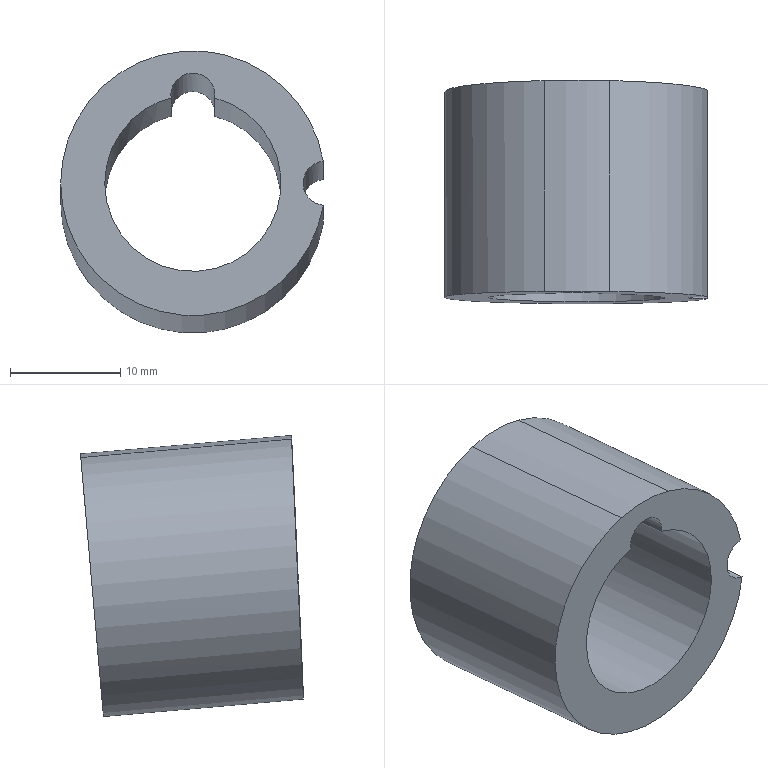Part | NX | features solid 2 | 1 solid | 8 faces | box 23.833 x 20.243 x 25.583 mm | volume 4465 mm3 | cylinder 5 | plane 2 | spline 1 | commonest cylinder face diameters 4 x2 24 x2 16 x1
STEP:
#1=CARTESIAN_POINT('',(201.703,-46.311,-35.578));
#2=VERTEX_POINT('',#1);
#3=CARTESIAN_POINT('',(210.56,-46.767,-45.207));
#4=VERTEX_POINT('',#3);
#5=CARTESIAN_POINT('',(198.727,-46.835,-47.202));
#6=DIRECTION('',(0.001957,0.999,-0.04546));
#7=DIRECTION('',(0.04675,0.04532,0.9979));
#8=AXIS2_PLACEMENT_3D('',#5,#6,#7);
#9=ELLIPSE('',#8,12.011,12.);
#10=EDGE_CURVE('',#2,#4,#9,.T.);
#11=ORIENTED_EDGE('',*,*,#10,.T.);
#12=CARTESIAN_POINT('',(210.56,-28.01,-46.848));
#13=VERTEX_POINT('',#12);
#14=CARTESIAN_POINT('',(210.56,-37.445,-46.023));
#15=DIRECTION('',(0.,0.9962,-0.08716));
#16=VECTOR('',#15,1000.);
#17=LINE('',#14,#16);
#18=EDGE_CURVE('',#4,#13,#17,.T.);
#19=ORIENTED_EDGE('',*,*,#18,.T.);
#20=CARTESIAN_POINT('',(201.703,-27.17,-37.253));
#21=VERTEX_POINT('',#20);
#22=CARTESIAN_POINT('',(198.727,-28.184,-48.834));
#23=DIRECTION('',(0.,0.9962,-0.08716));
#24=DIRECTION('',(0.,0.08716,0.9962));
#25=AXIS2_PLACEMENT_3D('',#22,#23,#24);
#26=CIRCLE('',#25,12.);
#27=EDGE_CURVE('',#21,#13,#26,.T.);
#28=ORIENTED_EDGE('',*,*,#27,.F.);
#29=CARTESIAN_POINT('',(201.703,-27.17,-37.253));
#30=DIRECTION('',(0.,-0.9962,0.08716));
#31=VECTOR('',#30,1000.);
#32=LINE('',#29,#31);
#33=EDGE_CURVE('',#21,#2,#32,.T.);
#34=ORIENTED_EDGE('',*,*,#33,.T.);
#35=EDGE_LOOP('',(#11,#19,#28,#34));
#36=FACE_BOUND('',#35,.T.);
#37=CARTESIAN_POINT('',(198.727,-28.184,-48.834));
#38=DIRECTION('',(0.,-0.9962,0.08716));
#39=DIRECTION('',(0.,-0.08716,-0.9962));
#40=AXIS2_PLACEMENT_3D('',#37,#38,#39);
#41=CYLINDRICAL_SURFACE('',#40,12.);
#42=ADVANCED_FACE('',(#36),#41,.T.);
#43=CARTESIAN_POINT('',(200.711,-46.486,-39.453));
#44=VERTEX_POINT('',#43);
#45=CARTESIAN_POINT('',(196.742,-46.478,-39.454));
#46=VERTEX_POINT('',#45);
#47=CARTESIAN_POINT('',(198.727,-46.835,-47.202));
#48=DIRECTION('',(0.001957,0.999,-0.04546));
#49=DIRECTION('',(0.04675,0.04532,0.9979));
#50=AXIS2_PLACEMENT_3D('',#47,#48,#49);
#51=ELLIPSE('',#50,8.007,8.);
#52=EDGE_CURVE('',#44,#46,#51,.T.);
#53=ORIENTED_EDGE('',*,*,#52,.F.);
#54=CARTESIAN_POINT('',(200.711,-27.508,-41.113));
#55=VERTEX_POINT('',#54);
#56=CARTESIAN_POINT('',(200.711,-27.508,-41.113));
#57=DIRECTION('',(0.,-0.9962,0.08716));
#58=VECTOR('',#57,1000.);
#59=LINE('',#56,#58);
#60=EDGE_CURVE('',#44,#55,#59,.F.);
#61=ORIENTED_EDGE('',*,*,#60,.T.);
#62=CARTESIAN_POINT('',(196.742,-27.508,-41.113));
#63=VERTEX_POINT('',#62);
#64=CARTESIAN_POINT('',(198.727,-28.184,-48.834));
#65=DIRECTION('',(0.,-0.9962,0.08716));
#66=DIRECTION('',(0.,-0.08716,-0.9962));
#67=AXIS2_PLACEMENT_3D('',#64,#65,#66);
#68=CIRCLE('',#67,8.);
#69=EDGE_CURVE('',#55,#63,#68,.F.);
#70=ORIENTED_EDGE('',*,*,#69,.T.);
#71=CARTESIAN_POINT('',(196.742,-27.508,-41.113));
#72=DIRECTION('',(0.,-0.9962,0.08716));
#73=VECTOR('',#72,1000.);
#74=LINE('',#71,#73);
#75=EDGE_CURVE('',#63,#46,#74,.T.);
#76=ORIENTED_EDGE('',*,*,#75,.T.);
#77=EDGE_LOOP('',(#53,#61,#70,#76));
#78=FACE_BOUND('',#77,.T.);
#79=CARTESIAN_POINT('',(198.727,-28.184,-48.834));
#80=DIRECTION('',(0.,-0.9962,0.08716));
#81=DIRECTION('',(0.,-0.08716,-0.9962));
#82=AXIS2_PLACEMENT_3D('',#79,#80,#81);
#83=CYLINDRICAL_SURFACE('',#82,8.);
#84=ADVANCED_FACE('',(#78),#83,.F.);
#85=CARTESIAN_POINT('',(210.56,-28.357,-50.819));
#86=VERTEX_POINT('',#85);
#87=CARTESIAN_POINT('',(210.727,-28.184,-48.834));
#88=DIRECTION('',(0.,-0.9962,0.08716));
#89=DIRECTION('',(0.,-0.08716,-0.9962));
#90=AXIS2_PLACEMENT_3D('',#87,#88,#89);
#91=CIRCLE('',#90,2.);
#92=EDGE_CURVE('',#13,#86,#91,.T.);
#93=ORIENTED_EDGE('',*,*,#92,.T.);
#94=CARTESIAN_POINT('',(195.75,-27.17,-37.253));
#95=VERTEX_POINT('',#94);
#96=CARTESIAN_POINT('',(198.727,-28.184,-48.834));
#97=DIRECTION('',(0.,0.9962,-0.08716));
#98=DIRECTION('',(0.,0.08716,0.9962));
#99=AXIS2_PLACEMENT_3D('',#96,#97,#98);
#100=CIRCLE('',#99,12.);
#101=EDGE_CURVE('',#86,#95,#100,.T.);
#102=ORIENTED_EDGE('',*,*,#101,.T.);
#103=CARTESIAN_POINT('',(195.75,-27.17,-37.253));
#104=CARTESIAN_POINT('',(197.703,-27.127,-36.755));
#105=CARTESIAN_POINT('',(199.75,-27.127,-36.755));
#106=CARTESIAN_POINT('',(201.703,-27.17,-37.253));
#107=B_SPLINE_CURVE_WITH_KNOTS('',3,(#103,#104,#105,#106),.UNSPECIFIED.,.F.,.F.,(4,4),(0.,1.),.PIECEWISE_BEZIER_KNOTS.);
#108=EDGE_CURVE('',#95,#21,#107,.T.);
#109=ORIENTED_EDGE('',*,*,#108,.T.);
#110=ORIENTED_EDGE('',*,*,#27,.T.);
#111=EDGE_LOOP('',(#93,#102,#109,#110));
#112=FACE_BOUND('',#111,.T.);
#113=CARTESIAN_POINT('',(198.727,-27.486,-40.864));
#114=DIRECTION('',(0.,-0.9962,0.08716));
#115=DIRECTION('',(0.,-0.08716,-0.9962));
#116=AXIS2_PLACEMENT_3D('',#113,#114,#115);
#117=CIRCLE('',#116,2.);
#118=EDGE_CURVE('',#55,#63,#117,.T.);
#119=ORIENTED_EDGE('',*,*,#118,.T.);
#120=ORIENTED_EDGE('',*,*,#69,.F.);
#121=EDGE_LOOP('',(#119,#120));
#122=FACE_BOUND('',#121,.T.);
#123=CARTESIAN_POINT('',(195.75,-27.17,-37.253));
#124=DIRECTION('',(0.,0.9962,-0.08716));
#125=DIRECTION('',(0.,0.08716,0.9962));
#126=AXIS2_PLACEMENT_3D('',#123,#124,#125);
#127=PLANE('',#126);
#128=ADVANCED_FACE('',(#112,#122),#127,.T.);
#129=CARTESIAN_POINT('',(210.56,-46.948,-49.193));
#130=VERTEX_POINT('',#129);
#131=CARTESIAN_POINT('',(210.727,-46.858,-47.2));
#132=DIRECTION('',(0.001957,0.999,-0.04546));
#133=DIRECTION('',(-0.04675,-0.04532,-0.9979));
#134=AXIS2_PLACEMENT_3D('',#131,#132,#133);
#135=ELLIPSE('',#134,2.002,2.);
#136=EDGE_CURVE('',#130,#4,#135,.T.);
#137=ORIENTED_EDGE('',*,*,#136,.T.);
#138=ORIENTED_EDGE('',*,*,#10,.F.);
#139=CARTESIAN_POINT('',(195.75,-46.3,-35.579));
#140=VERTEX_POINT('',#139);
#141=CARTESIAN_POINT('',(195.75,-46.3,-35.579));
#142=CARTESIAN_POINT('',(197.699,-46.281,-35.08));
#143=CARTESIAN_POINT('',(199.754,-46.285,-35.08));
#144=CARTESIAN_POINT('',(201.703,-46.311,-35.578));
#145=B_SPLINE_CURVE_WITH_KNOTS('',3,(#141,#142,#143,#144),.UNSPECIFIED.,.F.,.F.,(4,4),(0.,0.006022),.UNSPECIFIED.);
#146=EDGE_CURVE('',#140,#2,#145,.T.);
#147=ORIENTED_EDGE('',*,*,#146,.F.);
#148=CARTESIAN_POINT('',(198.727,-46.835,-47.202));
#149=DIRECTION('',(0.001957,0.999,-0.04546));
#150=DIRECTION('',(0.04675,0.04532,0.9979));
#151=AXIS2_PLACEMENT_3D('',#148,#149,#150);
#152=ELLIPSE('',#151,12.011,12.);
#153=EDGE_CURVE('',#130,#140,#152,.T.);
#154=ORIENTED_EDGE('',*,*,#153,.F.);
#155=EDGE_LOOP('',(#137,#138,#147,#154));
#156=FACE_BOUND('',#155,.T.);
#157=CARTESIAN_POINT('',(198.727,-46.471,-39.203));
#158=DIRECTION('',(0.001957,0.999,-0.04546));
#159=DIRECTION('',(-0.04675,-0.04532,-0.9979));
#160=AXIS2_PLACEMENT_3D('',#157,#158,#159);
#161=ELLIPSE('',#160,2.002,2.);
#162=EDGE_CURVE('',#46,#44,#161,.T.);
#163=ORIENTED_EDGE('',*,*,#162,.T.);
#164=ORIENTED_EDGE('',*,*,#52,.T.);
#165=EDGE_LOOP('',(#163,#164));
#166=FACE_BOUND('',#165,.T.);
#167=CARTESIAN_POINT('',(128.811,-48.589,-88.763));
#168=DIRECTION('',(0.001957,0.999,-0.04546));
#169=DIRECTION('',(0.06617,0.04523,0.9968));
#170=AXIS2_PLACEMENT_3D('',#167,#168,#169);
#171=PLANE('',#170);
#172=ADVANCED_FACE('',(#156,#166),#171,.F.);
#173=ORIENTED_EDGE('',*,*,#101,.F.);
#174=CARTESIAN_POINT('',(210.56,-37.792,-49.994));
#175=DIRECTION('',(0.,0.9962,-0.08716));
#176=VECTOR('',#175,1000.);
#177=LINE('',#174,#176);
#178=EDGE_CURVE('',#86,#130,#177,.F.);
#179=ORIENTED_EDGE('',*,*,#178,.T.);
#180=ORIENTED_EDGE('',*,*,#153,.T.);
#181=CARTESIAN_POINT('',(195.75,-27.17,-37.253));
#182=DIRECTION('',(0.,-0.9962,0.08716));
#183=VECTOR('',#182,1000.);
#184=LINE('',#181,#183);
#185=EDGE_CURVE('',#95,#140,#184,.T.);
#186=ORIENTED_EDGE('',*,*,#185,.F.);
#187=EDGE_LOOP('',(#173,#179,#180,#186));
#188=FACE_BOUND('',#187,.T.);
#189=CARTESIAN_POINT('',(198.727,-28.184,-48.834));
#190=DIRECTION('',(0.,-0.9962,0.08716));
#191=DIRECTION('',(0.,-0.08716,-0.9962));
#192=AXIS2_PLACEMENT_3D('',#189,#190,#191);
#193=CYLINDRICAL_SURFACE('',#192,12.);
#194=ADVANCED_FACE('',(#188),#193,.T.);
#195=ORIENTED_EDGE('',*,*,#146,.T.);
#196=ORIENTED_EDGE('',*,*,#33,.F.);
#197=ORIENTED_EDGE('',*,*,#108,.F.);
#198=ORIENTED_EDGE('',*,*,#185,.T.);
#199=EDGE_LOOP('',(#195,#196,#197,#198));
#200=FACE_BOUND('',#199,.T.);
#201=CARTESIAN_POINT('',(195.75,-27.17,-37.253));
#202=CARTESIAN_POINT('',(195.75,-46.438,-35.567));
#203=CARTESIAN_POINT('',(197.703,-27.127,-36.755));
#204=CARTESIAN_POINT('',(197.703,-46.394,-35.069));
#205=CARTESIAN_POINT('',(199.75,-27.127,-36.755));
#206=CARTESIAN_POINT('',(199.75,-46.394,-35.069));
#207=CARTESIAN_POINT('',(201.703,-27.17,-37.253));
#208=CARTESIAN_POINT('',(201.703,-46.438,-35.567));
#209=B_SPLINE_SURFACE_WITH_KNOTS('',3,1,((#201,#202),(#203,#204),(#205,#206),(#207,#208)),.SURF_OF_LINEAR_EXTRUSION.,.F.,.F.,.F.,(4,4),(2,2),(0.,1.),(0.,1.),.PIECEWISE_BEZIER_KNOTS.);
#210=ADVANCED_FACE('',(#200),#209,.F.);
#211=ORIENTED_EDGE('',*,*,#75,.F.);
#212=ORIENTED_EDGE('',*,*,#118,.F.);
#213=ORIENTED_EDGE('',*,*,#60,.F.);
#214=ORIENTED_EDGE('',*,*,#162,.F.);
#215=EDGE_LOOP('',(#211,#212,#213,#214));
#216=FACE_BOUND('',#215,.T.);
#217=CARTESIAN_POINT('',(198.727,-47.41,-39.121));
#218=DIRECTION('',(0.,0.9962,-0.08716));
#219=DIRECTION('',(0.,0.08716,0.9962));
#220=AXIS2_PLACEMENT_3D('',#217,#218,#219);
#221=CYLINDRICAL_SURFACE('',#220,2.);
#222=ADVANCED_FACE('',(#216),#221,.F.);
#223=ORIENTED_EDGE('',*,*,#136,.F.);
#224=ORIENTED_EDGE('',*,*,#178,.F.);
#225=ORIENTED_EDGE('',*,*,#92,.F.);
#226=ORIENTED_EDGE('',*,*,#18,.F.);
#227=EDGE_LOOP('',(#223,#224,#225,#226));
#228=FACE_BOUND('',#227,.T.);
#229=CARTESIAN_POINT('',(210.727,-48.107,-47.091));
#230=DIRECTION('',(0.,0.9962,-0.08716));
#231=DIRECTION('',(0.,0.08716,0.9962));
#232=AXIS2_PLACEMENT_3D('',#229,#230,#231);
#233=CYLINDRICAL_SURFACE('',#232,2.);
#234=ADVANCED_FACE('',(#228),#233,.F.);
#235=CLOSED_SHELL('',(#42,#84,#128,#172,#194,#210,#222,#234));
#236=MANIFOLD_SOLID_BREP('',#235);
#237=(LENGTH_UNIT()NAMED_UNIT(*)SI_UNIT(.MILLI.,.METRE.));
#238=UNCERTAINTY_MEASURE_WITH_UNIT(LENGTH_MEASURE(0.0508),#237,'','');
#239=(NAMED_UNIT(*)PLANE_ANGLE_UNIT()SI_UNIT($,.RADIAN.));
#240=(NAMED_UNIT(*)SI_UNIT($,.STERADIAN.)SOLID_ANGLE_UNIT());
#241=(GEOMETRIC_REPRESENTATION_CONTEXT(3)GLOBAL_UNCERTAINTY_ASSIGNED_CONTEXT((#238))GLOBAL_UNIT_ASSIGNED_CONTEXT((#237,#239,#240))REPRESENTATION_CONTEXT('',''));
#242=ADVANCED_BREP_SHAPE_REPRESENTATION('',(#236),#241);